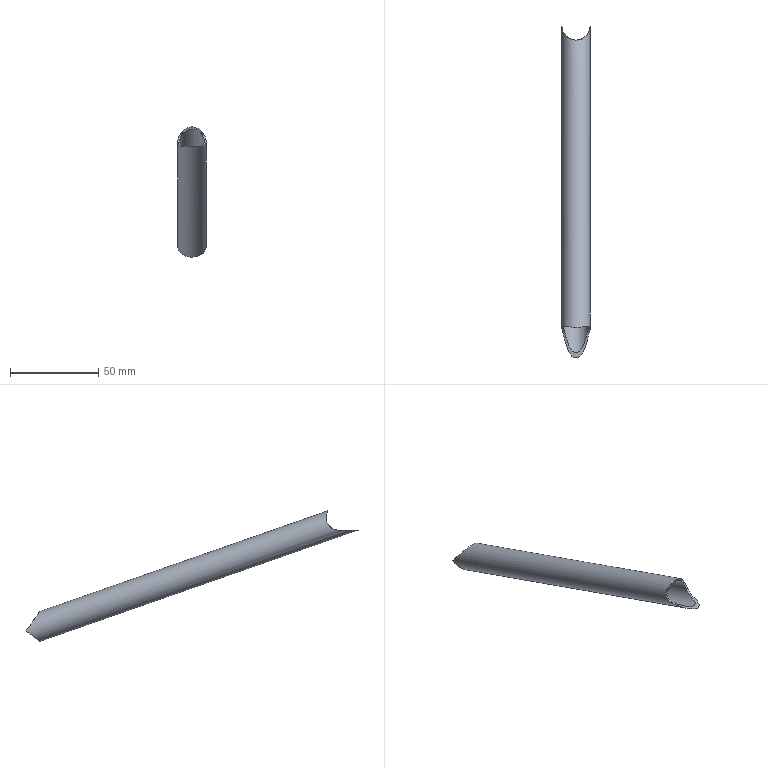Part | NX | features MG0313 aframe 2 | 1 solid | 9 faces | box 15.875 x 187.806 x 73.648 mm | volume 8495 mm3 | cylinder 6 | plane 3 | commonest cylinder face diameters 13.31 x3 15.875 x2 13.843 x1